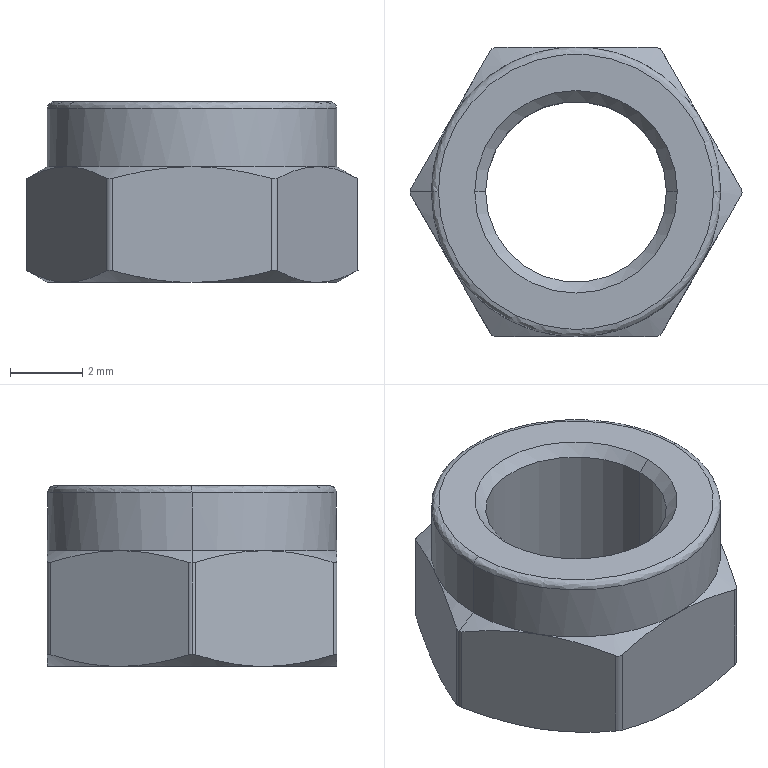Part | SolidWorks | features BaseBody 1 | 1 solid | 39 faces | box 9.176 x 8 x 5 mm | volume 166.809 mm3 | cone 18 | cylinder 11 | plane 8 | spline 2 | commonest cylinder face diameters 0.4 x7 5 x2 8 x2
STEP:
#1=CARTESIAN_POINT('',(-3.8,0.,5.));
#2=VERTEX_POINT('',#1);
#3=CARTESIAN_POINT('',(3.8,0.,5.));
#4=VERTEX_POINT('',#3);
#5=CARTESIAN_POINT('',(-3.8,0.,5.));
#6=CARTESIAN_POINT('',(-3.8,-0.2415,5.));
#7=CARTESIAN_POINT('',(-3.767,-0.5975,5.));
#8=CARTESIAN_POINT('',(-3.669,-1.002,5.));
#9=CARTESIAN_POINT('',(-3.606,-1.201,5.));
#10=CARTESIAN_POINT('',(-3.576,-1.286,5.));
#11=CARTESIAN_POINT('',(-3.555,-1.343,5.));
#12=CARTESIAN_POINT('',(-3.545,-1.369,5.));
#13=CARTESIAN_POINT('',(-3.486,-1.518,5.));
#14=CARTESIAN_POINT('',(-3.407,-1.693,5.));
#15=CARTESIAN_POINT('',(-3.314,-1.86,5.));
#16=CARTESIAN_POINT('',(-3.249,-1.971,5.));
#17=CARTESIAN_POINT('',(-3.216,-2.025,5.));
#18=CARTESIAN_POINT('',(-3.037,-2.299,5.));
#19=CARTESIAN_POINT('',(-2.872,-2.502,5.));
#20=CARTESIAN_POINT('',(-2.594,-2.78,5.));
#21=CARTESIAN_POINT('',(-2.449,-2.911,5.));
#22=CARTESIAN_POINT('',(-2.294,-3.03,5.));
#23=CARTESIAN_POINT('',(-2.188,-3.107,5.));
#24=CARTESIAN_POINT('',(-2.133,-3.145,5.));
#25=CARTESIAN_POINT('',(-1.972,-3.251,5.));
#26=CARTESIAN_POINT('',(-1.806,-3.347,5.));
#27=CARTESIAN_POINT('',(-1.605,-3.445,5.));
#28=CARTESIAN_POINT('',(-1.517,-3.484,5.));
#29=CARTESIAN_POINT('',(-1.458,-3.509,5.));
#30=CARTESIAN_POINT('',(-1.427,-3.522,5.));
#31=CARTESIAN_POINT('',(-0.9498,-3.711,5.));
#32=CARTESIAN_POINT('',(-0.4829,-3.8,5.));
#33=CARTESIAN_POINT('',(0.2414,-3.8,5.));
#34=CARTESIAN_POINT('',(0.5974,-3.767,5.));
#35=CARTESIAN_POINT('',(1.002,-3.669,5.));
#36=CARTESIAN_POINT('',(1.201,-3.606,5.));
#37=CARTESIAN_POINT('',(1.286,-3.576,5.));
#38=CARTESIAN_POINT('',(1.342,-3.555,5.));
#39=CARTESIAN_POINT('',(1.369,-3.545,5.));
#40=CARTESIAN_POINT('',(1.518,-3.486,5.));
#41=CARTESIAN_POINT('',(1.693,-3.407,5.));
#42=CARTESIAN_POINT('',(1.86,-3.314,5.));
#43=CARTESIAN_POINT('',(1.971,-3.249,5.));
#44=CARTESIAN_POINT('',(2.025,-3.216,5.));
#45=CARTESIAN_POINT('',(2.299,-3.037,5.));
#46=CARTESIAN_POINT('',(2.502,-2.872,5.));
#47=CARTESIAN_POINT('',(2.78,-2.594,5.));
#48=CARTESIAN_POINT('',(2.911,-2.449,5.));
#49=CARTESIAN_POINT('',(3.03,-2.294,5.));
#50=CARTESIAN_POINT('',(3.107,-2.188,5.));
#51=CARTESIAN_POINT('',(3.145,-2.133,5.));
#52=CARTESIAN_POINT('',(3.251,-1.972,5.));
#53=CARTESIAN_POINT('',(3.347,-1.806,5.));
#54=CARTESIAN_POINT('',(3.445,-1.605,5.));
#55=CARTESIAN_POINT('',(3.484,-1.517,5.));
#56=CARTESIAN_POINT('',(3.509,-1.458,5.));
#57=CARTESIAN_POINT('',(3.522,-1.427,5.));
#58=CARTESIAN_POINT('',(3.711,-0.9496,5.));
#59=CARTESIAN_POINT('',(3.8,-0.4834,5.));
#60=CARTESIAN_POINT('',(3.8,0.,5.));
#61=B_SPLINE_CURVE_WITH_KNOTS('',3,(#5,#6,#7,#8,#9,#10,#11,#12,#13,#14,#15,#16,#17,#18,#19,#20,#21,#22,#23,#24,#25,#26,#27,#28,#29,#30,#31,#32,#33,#34,#35,#36,#37,#38,#39,#40,#41,#42,#43,#44,#45,#46,#47,#48,#49,#50,#51,#52,#53,#54,#55,#56,#57,#58,#59,#60),.UNSPECIFIED.,.F.,.F.,(4,1,1,1,2,2,1,2,2,2,1,2,2,1,1,2,2,2,1,1,1,2,2,1,2,2,2,1,2,2,1,1,2,2,4),(0.,0.0625,0.09375,0.1094,0.1172,0.125,0.1562,0.1719,0.1875,0.25,0.2812,0.2969,0.3125,0.3437,0.3594,0.3672,0.375,0.5,0.5625,0.5937,0.6094,0.6172,0.625,0.6562,0.6719,0.6875,0.75,0.7812,0.7969,0.8125,0.8437,0.8594,0.8672,0.875,1.),.UNSPECIFIED.);
#62=EDGE_CURVE('',#2,#4,#61,.T.);
#63=ORIENTED_EDGE('',*,*,#62,.F.);
#64=CARTESIAN_POINT('',(-4.,0.,4.8));
#65=VERTEX_POINT('',#64);
#66=CARTESIAN_POINT('',(-3.8,0.,4.8));
#67=DIRECTION('',(0.,-1.,0.));
#68=DIRECTION('',(-1.,0.,0.));
#69=AXIS2_PLACEMENT_3D('',#66,#67,#68);
#70=CIRCLE('',#69,0.2);
#71=EDGE_CURVE('',#2,#65,#70,.T.);
#72=ORIENTED_EDGE('',*,*,#71,.T.);
#73=CARTESIAN_POINT('',(4.,0.,4.8));
#74=VERTEX_POINT('',#73);
#75=CARTESIAN_POINT('',(0.,0.,4.8));
#76=DIRECTION('',(0.,0.,1.));
#77=DIRECTION('',(1.,0.,0.));
#78=AXIS2_PLACEMENT_3D('',#75,#76,#77);
#79=CIRCLE('',#78,4.);
#80=EDGE_CURVE('',#65,#74,#79,.T.);
#81=ORIENTED_EDGE('',*,*,#80,.T.);
#82=CARTESIAN_POINT('',(3.8,0.,4.8));
#83=DIRECTION('',(0.,1.,0.));
#84=DIRECTION('',(1.,0.,0.));
#85=AXIS2_PLACEMENT_3D('',#82,#83,#84);
#86=CIRCLE('',#85,0.2);
#87=EDGE_CURVE('',#4,#74,#86,.T.);
#88=ORIENTED_EDGE('',*,*,#87,.F.);
#89=EDGE_LOOP('',(#63,#72,#81,#88));
#90=FACE_OUTER_BOUND('',#89,.T.);
#91=CARTESIAN_POINT('',(-3.8,0.,5.));
#92=CARTESIAN_POINT('',(-3.8,-7.6,5.));
#93=CARTESIAN_POINT('',(3.8,-7.6,5.));
#94=CARTESIAN_POINT('',(3.8,0.,5.));
#95=CARTESIAN_POINT('',(-3.917,0.,5.));
#96=CARTESIAN_POINT('',(-3.917,-7.834,5.));
#97=CARTESIAN_POINT('',(3.917,-7.834,5.));
#98=CARTESIAN_POINT('',(3.917,0.,5.));
#99=CARTESIAN_POINT('',(-4.,0.,4.917));
#100=CARTESIAN_POINT('',(-4.,-8.,4.917));
#101=CARTESIAN_POINT('',(4.,-8.,4.917));
#102=CARTESIAN_POINT('',(4.,0.,4.917));
#103=CARTESIAN_POINT('',(-4.,0.,4.8));
#104=CARTESIAN_POINT('',(-4.,-8.,4.8));
#105=CARTESIAN_POINT('',(4.,-8.,4.8));
#106=CARTESIAN_POINT('',(4.,0.,4.8));
#107=(BOUNDED_SURFACE()B_SPLINE_SURFACE(3,3,((#91,#92,#93,#94),(#95,#96,#97,#98),(#99,#100,#101,#102),(#103,#104,#105,#106)),.UNSPECIFIED.,.F.,.F.,.T.)B_SPLINE_SURFACE_WITH_KNOTS((4,4),(4,4),(0.,1.),(0.,1.),.UNSPECIFIED.)GEOMETRIC_REPRESENTATION_ITEM()RATIONAL_B_SPLINE_SURFACE(((1.,0.3333,0.3333,1.),(0.8047,0.2682,0.2682,0.8047),(0.8047,0.2682,0.2682,0.8047),(1.,0.3333,0.3333,1.)))REPRESENTATION_ITEM('')SURFACE());
#108=ADVANCED_FACE('',(#90),#107,.T.);
#109=CARTESIAN_POINT('',(-2.5,0.,0.3));
#110=VERTEX_POINT('',#109);
#111=CARTESIAN_POINT('',(2.5,0.,0.3));
#112=VERTEX_POINT('',#111);
#113=CARTESIAN_POINT('',(0.,0.,0.3));
#114=DIRECTION('',(0.,0.,1.));
#115=DIRECTION('',(1.,0.,0.));
#116=AXIS2_PLACEMENT_3D('',#113,#114,#115);
#117=CIRCLE('',#116,2.5);
#118=EDGE_CURVE('',#110,#112,#117,.T.);
#119=ORIENTED_EDGE('',*,*,#118,.F.);
#120=CARTESIAN_POINT('',(-2.5,0.,4.7));
#121=VERTEX_POINT('',#120);
#122=CARTESIAN_POINT('',(-2.5,0.,0.));
#123=DIRECTION('',(0.,0.,1.));
#124=VECTOR('',#123,1000.);
#125=LINE('',#122,#124);
#126=EDGE_CURVE('',#110,#121,#125,.T.);
#127=ORIENTED_EDGE('',*,*,#126,.T.);
#128=CARTESIAN_POINT('',(2.5,0.,4.7));
#129=VERTEX_POINT('',#128);
#130=CARTESIAN_POINT('',(0.,0.,4.7));
#131=DIRECTION('',(0.,0.,-1.));
#132=DIRECTION('',(1.,0.,0.));
#133=AXIS2_PLACEMENT_3D('',#130,#131,#132);
#134=CIRCLE('',#133,2.5);
#135=EDGE_CURVE('',#129,#121,#134,.T.);
#136=ORIENTED_EDGE('',*,*,#135,.F.);
#137=CARTESIAN_POINT('',(2.5,0.,0.));
#138=DIRECTION('',(0.,0.,1.));
#139=VECTOR('',#138,1000.);
#140=LINE('',#137,#139);
#141=EDGE_CURVE('',#112,#129,#140,.T.);
#142=ORIENTED_EDGE('',*,*,#141,.F.);
#143=EDGE_LOOP('',(#119,#127,#136,#142));
#144=FACE_OUTER_BOUND('',#143,.T.);
#145=CARTESIAN_POINT('',(0.,0.,0.));
#146=DIRECTION('',(0.,0.,1.));
#147=DIRECTION('',(1.,0.,0.));
#148=AXIS2_PLACEMENT_3D('',#145,#146,#147);
#149=CYLINDRICAL_SURFACE('',#148,2.5);
#150=ADVANCED_FACE('',(#144),#149,.F.);
#151=ORIENTED_EDGE('',*,*,#118,.T.);
#152=CARTESIAN_POINT('',(2.8,0.,0.));
#153=VERTEX_POINT('',#152);
#154=CARTESIAN_POINT('',(2.8,0.,0.));
#155=DIRECTION('',(0.7071,0.,-0.7071));
#156=VECTOR('',#155,1000.);
#157=LINE('',#154,#156);
#158=EDGE_CURVE('',#112,#153,#157,.T.);
#159=ORIENTED_EDGE('',*,*,#158,.T.);
#160=CARTESIAN_POINT('',(-2.8,0.,0.));
#161=VERTEX_POINT('',#160);
#162=CARTESIAN_POINT('',(0.,0.,0.));
#163=DIRECTION('',(0.,0.,1.));
#164=DIRECTION('',(-1.,0.,0.));
#165=AXIS2_PLACEMENT_3D('',#162,#163,#164);
#166=CIRCLE('',#165,2.8);
#167=EDGE_CURVE('',#161,#153,#166,.T.);
#168=ORIENTED_EDGE('',*,*,#167,.F.);
#169=CARTESIAN_POINT('',(-2.8,0.,0.));
#170=DIRECTION('',(-0.7071,0.,-0.7071));
#171=VECTOR('',#170,1000.);
#172=LINE('',#169,#171);
#173=EDGE_CURVE('',#110,#161,#172,.T.);
#174=ORIENTED_EDGE('',*,*,#173,.F.);
#175=EDGE_LOOP('',(#151,#159,#168,#174));
#176=FACE_OUTER_BOUND('',#175,.T.);
#177=CARTESIAN_POINT('',(0.,0.,0.));
#178=DIRECTION('',(0.,0.,-1.));
#179=DIRECTION('',(-1.,0.,0.));
#180=AXIS2_PLACEMENT_3D('',#177,#178,#179);
#181=CONICAL_SURFACE('',#180,2.8,0.7854);
#182=ADVANCED_FACE('',(#176),#181,.F.);
#183=ORIENTED_EDGE('',*,*,#135,.T.);
#184=CARTESIAN_POINT('',(-2.8,0.,5.));
#185=VERTEX_POINT('',#184);
#186=CARTESIAN_POINT('',(-2.8,0.,5.));
#187=DIRECTION('',(-0.7071,0.,0.7071));
#188=VECTOR('',#187,1000.);
#189=LINE('',#186,#188);
#190=EDGE_CURVE('',#121,#185,#189,.T.);
#191=ORIENTED_EDGE('',*,*,#190,.T.);
#192=CARTESIAN_POINT('',(2.8,0.,5.));
#193=VERTEX_POINT('',#192);
#194=CARTESIAN_POINT('',(0.,0.,5.));
#195=DIRECTION('',(0.,0.,-1.));
#196=DIRECTION('',(1.,0.,0.));
#197=AXIS2_PLACEMENT_3D('',#194,#195,#196);
#198=CIRCLE('',#197,2.8);
#199=EDGE_CURVE('',#193,#185,#198,.T.);
#200=ORIENTED_EDGE('',*,*,#199,.F.);
#201=CARTESIAN_POINT('',(2.8,0.,5.));
#202=DIRECTION('',(0.7071,0.,0.7071));
#203=VECTOR('',#202,1000.);
#204=LINE('',#201,#203);
#205=EDGE_CURVE('',#129,#193,#204,.T.);
#206=ORIENTED_EDGE('',*,*,#205,.F.);
#207=EDGE_LOOP('',(#183,#191,#200,#206));
#208=FACE_OUTER_BOUND('',#207,.T.);
#209=CARTESIAN_POINT('',(0.,0.,5.));
#210=DIRECTION('',(0.,0.,1.));
#211=DIRECTION('',(1.,0.,0.));
#212=AXIS2_PLACEMENT_3D('',#209,#210,#211);
#213=CONICAL_SURFACE('',#212,2.8,0.7854);
#214=ADVANCED_FACE('',(#208),#213,.F.);
#215=CARTESIAN_POINT('',(3.464,-2.,0.));
#216=VERTEX_POINT('',#215);
#217=CARTESIAN_POINT('',(4.,0.,0.));
#218=VERTEX_POINT('',#217);
#219=CARTESIAN_POINT('',(0.,0.,0.));
#220=DIRECTION('',(0.,0.,1.));
#221=DIRECTION('',(1.,0.,0.));
#222=AXIS2_PLACEMENT_3D('',#219,#220,#221);
#223=CIRCLE('',#222,4.);
#224=EDGE_CURVE('',#216,#218,#223,.T.);
#225=ORIENTED_EDGE('',*,*,#224,.T.);
#226=CARTESIAN_POINT('',(4.588,0.,0.3394));
#227=VERTEX_POINT('',#226);
#228=CARTESIAN_POINT('',(4.591,0.,0.3414));
#229=DIRECTION('',(0.866,0.,0.5));
#230=VECTOR('',#229,1000.);
#231=LINE('',#228,#230);
#232=EDGE_CURVE('',#218,#227,#231,.T.);
#233=ORIENTED_EDGE('',*,*,#232,.T.);
#234=CARTESIAN_POINT('',(4.561,-0.1,0.3246));
#235=VERTEX_POINT('',#234);
#236=CARTESIAN_POINT('',(4.561,-0.1,0.3246));
#237=CARTESIAN_POINT('',(4.578,-0.07028,0.3341));
#238=CARTESIAN_POINT('',(4.588,-0.03564,0.3394));
#239=CARTESIAN_POINT('',(4.588,0.,0.3394));
#240=B_SPLINE_CURVE_WITH_KNOTS('',3,(#236,#237,#238,#239),.UNSPECIFIED.,.F.,.F.,(4,4),(-0.0001053,0.),.UNSPECIFIED.);
#241=EDGE_CURVE('',#235,#227,#240,.T.);
#242=ORIENTED_EDGE('',*,*,#241,.F.);
#243=CARTESIAN_POINT('',(4.561,-0.1,0.3246));
#244=CARTESIAN_POINT('',(4.202,-0.7217,0.1253));
#245=CARTESIAN_POINT('',(3.838,-1.353,0.));
#246=CARTESIAN_POINT('',(3.464,-2.,0.));
#247=B_SPLINE_CURVE_WITH_KNOTS('',3,(#243,#244,#245,#246),.UNSPECIFIED.,.F.,.F.,(4,4),(0.,0.002218),.UNSPECIFIED.);
#248=EDGE_CURVE('',#235,#216,#247,.T.);
#249=ORIENTED_EDGE('',*,*,#248,.T.);
#250=EDGE_LOOP('',(#225,#233,#242,#249));
#251=FACE_OUTER_BOUND('',#250,.T.);
#252=CARTESIAN_POINT('',(0.,0.,0.3414));
#253=DIRECTION('',(0.,0.,1.));
#254=DIRECTION('',(1.,0.,0.));
#255=AXIS2_PLACEMENT_3D('',#252,#253,#254);
#256=CONICAL_SURFACE('',#255,4.591,1.047);
#257=ADVANCED_FACE('',(#251),#256,.T.);
#258=CARTESIAN_POINT('',(0.,0.,4.8));
#259=DIRECTION('',(0.,0.,1.));
#260=DIRECTION('',(1.,0.,0.));
#261=AXIS2_PLACEMENT_3D('',#258,#259,#260);
#262=CIRCLE('',#261,4.);
#263=EDGE_CURVE('',#74,#65,#262,.T.);
#264=ORIENTED_EDGE('',*,*,#263,.F.);
#265=CARTESIAN_POINT('',(4.,0.,3.2));
#266=VERTEX_POINT('',#265);
#267=CARTESIAN_POINT('',(4.,0.,5.));
#268=DIRECTION('',(0.,0.,-1.));
#269=VECTOR('',#268,1000.);
#270=LINE('',#267,#269);
#271=EDGE_CURVE('',#74,#266,#270,.T.);
#272=ORIENTED_EDGE('',*,*,#271,.T.);
#273=CARTESIAN_POINT('',(3.464,2.,3.2));
#274=VERTEX_POINT('',#273);
#275=CARTESIAN_POINT('',(0.,0.,3.2));
#276=DIRECTION('',(0.,0.,1.));
#277=DIRECTION('',(-1.,0.,0.));
#278=AXIS2_PLACEMENT_3D('',#275,#276,#277);
#279=CIRCLE('',#278,4.);
#280=EDGE_CURVE('',#266,#274,#279,.T.);
#281=ORIENTED_EDGE('',*,*,#280,.T.);
#282=CARTESIAN_POINT('',(0.,4.,3.2));
#283=VERTEX_POINT('',#282);
#284=CARTESIAN_POINT('',(0.,0.,3.2));
#285=DIRECTION('',(0.,0.,1.));
#286=DIRECTION('',(-1.,0.,0.));
#287=AXIS2_PLACEMENT_3D('',#284,#285,#286);
#288=CIRCLE('',#287,4.);
#289=EDGE_CURVE('',#274,#283,#288,.T.);
#290=ORIENTED_EDGE('',*,*,#289,.T.);
#291=CARTESIAN_POINT('',(-3.464,2.,3.2));
#292=VERTEX_POINT('',#291);
#293=CARTESIAN_POINT('',(0.,0.,3.2));
#294=DIRECTION('',(0.,0.,1.));
#295=DIRECTION('',(-1.,0.,0.));
#296=AXIS2_PLACEMENT_3D('',#293,#294,#295);
#297=CIRCLE('',#296,4.);
#298=EDGE_CURVE('',#283,#292,#297,.T.);
#299=ORIENTED_EDGE('',*,*,#298,.T.);
#300=CARTESIAN_POINT('',(-4.,0.,3.2));
#301=VERTEX_POINT('',#300);
#302=CARTESIAN_POINT('',(0.,0.,3.2));
#303=DIRECTION('',(0.,0.,1.));
#304=DIRECTION('',(-1.,0.,0.));
#305=AXIS2_PLACEMENT_3D('',#302,#303,#304);
#306=CIRCLE('',#305,4.);
#307=EDGE_CURVE('',#292,#301,#306,.T.);
#308=ORIENTED_EDGE('',*,*,#307,.T.);
#309=CARTESIAN_POINT('',(-4.,0.,5.));
#310=DIRECTION('',(0.,0.,-1.));
#311=VECTOR('',#310,1000.);
#312=LINE('',#309,#311);
#313=EDGE_CURVE('',#65,#301,#312,.T.);
#314=ORIENTED_EDGE('',*,*,#313,.F.);
#315=EDGE_LOOP('',(#264,#272,#281,#290,#299,#308,#314));
#316=FACE_OUTER_BOUND('',#315,.T.);
#317=CARTESIAN_POINT('',(0.,0.,5.));
#318=DIRECTION('',(0.,0.,-1.));
#319=DIRECTION('',(-1.,0.,0.));
#320=AXIS2_PLACEMENT_3D('',#317,#318,#319);
#321=CYLINDRICAL_SURFACE('',#320,4.);
#322=ADVANCED_FACE('',(#316),#321,.T.);
#323=CARTESIAN_POINT('',(-3.464,-2.,3.2));
#324=VERTEX_POINT('',#323);
#325=CARTESIAN_POINT('',(0.,0.,3.2));
#326=DIRECTION('',(0.,0.,1.));
#327=DIRECTION('',(-1.,0.,0.));
#328=AXIS2_PLACEMENT_3D('',#325,#326,#327);
#329=CIRCLE('',#328,4.);
#330=EDGE_CURVE('',#301,#324,#329,.T.);
#331=ORIENTED_EDGE('',*,*,#330,.F.);
#332=CARTESIAN_POINT('',(-4.588,0.,2.861));
#333=VERTEX_POINT('',#332);
#334=CARTESIAN_POINT('',(-4.591,0.,2.859));
#335=DIRECTION('',(-0.866,0.,-0.5));
#336=VECTOR('',#335,1000.);
#337=LINE('',#334,#336);
#338=EDGE_CURVE('',#301,#333,#337,.T.);
#339=ORIENTED_EDGE('',*,*,#338,.T.);
#340=CARTESIAN_POINT('',(-4.561,-0.1,2.875));
#341=VERTEX_POINT('',#340);
#342=CARTESIAN_POINT('',(-4.588,0.,2.861));
#343=CARTESIAN_POINT('',(-4.588,-0.03565,2.861));
#344=CARTESIAN_POINT('',(-4.578,-0.07027,2.866));
#345=CARTESIAN_POINT('',(-4.561,-0.1,2.875));
#346=B_SPLINE_CURVE_WITH_KNOTS('',3,(#342,#343,#344,#345),.UNSPECIFIED.,.F.,.F.,(4,4),(0.,0.0001053),.UNSPECIFIED.);
#347=EDGE_CURVE('',#333,#341,#346,.T.);
#348=ORIENTED_EDGE('',*,*,#347,.T.);
#349=CARTESIAN_POINT('',(-4.561,-0.1,2.875));
#350=CARTESIAN_POINT('',(-4.202,-0.7217,3.075));
#351=CARTESIAN_POINT('',(-3.838,-1.353,3.2));
#352=CARTESIAN_POINT('',(-3.464,-2.,3.2));
#353=B_SPLINE_CURVE_WITH_KNOTS('',3,(#349,#350,#351,#352),.UNSPECIFIED.,.F.,.F.,(4,4),(0.,0.002218),.UNSPECIFIED.);
#354=EDGE_CURVE('',#341,#324,#353,.T.);
#355=ORIENTED_EDGE('',*,*,#354,.T.);
#356=EDGE_LOOP('',(#331,#339,#348,#355));
#357=FACE_OUTER_BOUND('',#356,.T.);
#358=CARTESIAN_POINT('',(0.,0.,2.859));
#359=DIRECTION('',(0.,0.,-1.));
#360=DIRECTION('',(-1.,0.,0.));
#361=AXIS2_PLACEMENT_3D('',#358,#359,#360);
#362=CONICAL_SURFACE('',#361,4.591,1.047);
#363=ADVANCED_FACE('',(#357),#362,.T.);
#364=ORIENTED_EDGE('',*,*,#347,.F.);
#365=CARTESIAN_POINT('',(-4.588,0.,0.3394));
#366=VERTEX_POINT('',#365);
#367=CARTESIAN_POINT('',(-4.588,0.,3.2));
#368=DIRECTION('',(0.,0.,-1.));
#369=VECTOR('',#368,1000.);
#370=LINE('',#367,#369);
#371=EDGE_CURVE('',#333,#366,#370,.T.);
#372=ORIENTED_EDGE('',*,*,#371,.T.);
#373=CARTESIAN_POINT('',(-4.561,-0.1,0.3246));
#374=VERTEX_POINT('',#373);
#375=CARTESIAN_POINT('',(-4.588,0.,0.3394));
#376=CARTESIAN_POINT('',(-4.588,-0.03565,0.3394));
#377=CARTESIAN_POINT('',(-4.578,-0.07027,0.3341));
#378=CARTESIAN_POINT('',(-4.561,-0.1,0.3246));
#379=B_SPLINE_CURVE_WITH_KNOTS('',3,(#375,#376,#377,#378),.UNSPECIFIED.,.F.,.F.,(4,4),(0.,0.0001053),.UNSPECIFIED.);
#380=EDGE_CURVE('',#366,#374,#379,.T.);
#381=ORIENTED_EDGE('',*,*,#380,.T.);
#382=CARTESIAN_POINT('',(-4.561,-0.1,3.2));
#383=DIRECTION('',(0.,0.,1.));
#384=VECTOR('',#383,1000.);
#385=LINE('',#382,#384);
#386=EDGE_CURVE('',#374,#341,#385,.T.);
#387=ORIENTED_EDGE('',*,*,#386,.T.);
#388=EDGE_LOOP('',(#364,#372,#381,#387));
#389=FACE_OUTER_BOUND('',#388,.T.);
#390=CARTESIAN_POINT('',(-4.388,0.,3.2));
#391=DIRECTION('',(0.,0.,-1.));
#392=DIRECTION('',(-1.,0.,0.));
#393=AXIS2_PLACEMENT_3D('',#390,#391,#392);
#394=CYLINDRICAL_SURFACE('',#393,0.2);
#395=ADVANCED_FACE('',(#389),#394,.T.);
#396=ORIENTED_EDGE('',*,*,#126,.F.);
#397=CARTESIAN_POINT('',(0.,0.,0.3));
#398=DIRECTION('',(0.,0.,1.));
#399=DIRECTION('',(1.,0.,0.));
#400=AXIS2_PLACEMENT_3D('',#397,#398,#399);
#401=CIRCLE('',#400,2.5);
#402=EDGE_CURVE('',#112,#110,#401,.T.);
#403=ORIENTED_EDGE('',*,*,#402,.F.);
#404=ORIENTED_EDGE('',*,*,#141,.T.);
#405=CARTESIAN_POINT('',(0.,0.,4.7));
#406=DIRECTION('',(0.,0.,-1.));
#407=DIRECTION('',(1.,0.,0.));
#408=AXIS2_PLACEMENT_3D('',#405,#406,#407);
#409=CIRCLE('',#408,2.5);
#410=EDGE_CURVE('',#121,#129,#409,.T.);
#411=ORIENTED_EDGE('',*,*,#410,.F.);
#412=EDGE_LOOP('',(#396,#403,#404,#411));
#413=FACE_OUTER_BOUND('',#412,.T.);
#414=CARTESIAN_POINT('',(0.,0.,0.));
#415=DIRECTION('',(0.,0.,1.));
#416=DIRECTION('',(1.,0.,0.));
#417=AXIS2_PLACEMENT_3D('',#414,#415,#416);
#418=CYLINDRICAL_SURFACE('',#417,2.5);
#419=ADVANCED_FACE('',(#413),#418,.F.);
#420=ORIENTED_EDGE('',*,*,#158,.F.);
#421=ORIENTED_EDGE('',*,*,#402,.T.);
#422=ORIENTED_EDGE('',*,*,#173,.T.);
#423=CARTESIAN_POINT('',(0.,0.,0.));
#424=DIRECTION('',(0.,0.,1.));
#425=DIRECTION('',(-1.,0.,0.));
#426=AXIS2_PLACEMENT_3D('',#423,#424,#425);
#427=CIRCLE('',#426,2.8);
#428=EDGE_CURVE('',#153,#161,#427,.T.);
#429=ORIENTED_EDGE('',*,*,#428,.F.);
#430=EDGE_LOOP('',(#420,#421,#422,#429));
#431=FACE_OUTER_BOUND('',#430,.T.);
#432=CARTESIAN_POINT('',(0.,0.,0.));
#433=DIRECTION('',(0.,0.,-1.));
#434=DIRECTION('',(-1.,0.,0.));
#435=AXIS2_PLACEMENT_3D('',#432,#433,#434);
#436=CONICAL_SURFACE('',#435,2.8,0.7854);
#437=ADVANCED_FACE('',(#431),#436,.F.);
#438=ORIENTED_EDGE('',*,*,#190,.F.);
#439=ORIENTED_EDGE('',*,*,#410,.T.);
#440=ORIENTED_EDGE('',*,*,#205,.T.);
#441=CARTESIAN_POINT('',(0.,0.,5.));
#442=DIRECTION('',(0.,0.,-1.));
#443=DIRECTION('',(1.,0.,0.));
#444=AXIS2_PLACEMENT_3D('',#441,#442,#443);
#445=CIRCLE('',#444,2.8);
#446=EDGE_CURVE('',#185,#193,#445,.T.);
#447=ORIENTED_EDGE('',*,*,#446,.F.);
#448=EDGE_LOOP('',(#438,#439,#440,#447));
#449=FACE_OUTER_BOUND('',#448,.T.);
#450=CARTESIAN_POINT('',(0.,0.,5.));
#451=DIRECTION('',(0.,0.,1.));
#452=DIRECTION('',(1.,0.,0.));
#453=AXIS2_PLACEMENT_3D('',#450,#451,#452);
#454=CONICAL_SURFACE('',#453,2.8,0.7854);
#455=ADVANCED_FACE('',(#449),#454,.F.);
#456=ORIENTED_EDGE('',*,*,#224,.F.);
#457=CARTESIAN_POINT('',(0.,-4.,0.));
#458=VERTEX_POINT('',#457);
#459=CARTESIAN_POINT('',(0.,0.,0.));
#460=DIRECTION('',(0.,0.,1.));
#461=DIRECTION('',(1.,0.,0.));
#462=AXIS2_PLACEMENT_3D('',#459,#460,#461);
#463=CIRCLE('',#462,4.);
#464=EDGE_CURVE('',#458,#216,#463,.T.);
#465=ORIENTED_EDGE('',*,*,#464,.F.);
#466=CARTESIAN_POINT('',(-3.464,-2.,0.));
#467=VERTEX_POINT('',#466);
#468=CARTESIAN_POINT('',(0.,0.,0.));
#469=DIRECTION('',(0.,0.,1.));
#470=DIRECTION('',(1.,0.,0.));
#471=AXIS2_PLACEMENT_3D('',#468,#469,#470);
#472=CIRCLE('',#471,4.);
#473=EDGE_CURVE('',#467,#458,#472,.T.);
#474=ORIENTED_EDGE('',*,*,#473,.F.);
#475=CARTESIAN_POINT('',(-3.464,2.,0.));
#476=VERTEX_POINT('',#475);
#477=CARTESIAN_POINT('',(0.,0.,0.));
#478=DIRECTION('',(0.,0.,1.));
#479=DIRECTION('',(1.,0.,0.));
#480=AXIS2_PLACEMENT_3D('',#477,#478,#479);
#481=CIRCLE('',#480,4.);
#482=EDGE_CURVE('',#476,#467,#481,.T.);
#483=ORIENTED_EDGE('',*,*,#482,.F.);
#484=CARTESIAN_POINT('',(0.,4.,0.));
#485=VERTEX_POINT('',#484);
#486=CARTESIAN_POINT('',(0.,0.,0.));
#487=DIRECTION('',(0.,0.,1.));
#488=DIRECTION('',(1.,0.,0.));
#489=AXIS2_PLACEMENT_3D('',#486,#487,#488);
#490=CIRCLE('',#489,4.);
#491=EDGE_CURVE('',#485,#476,#490,.T.);
#492=ORIENTED_EDGE('',*,*,#491,.F.);
#493=CARTESIAN_POINT('',(3.464,2.,0.));
#494=VERTEX_POINT('',#493);
#495=CARTESIAN_POINT('',(0.,0.,0.));
#496=DIRECTION('',(0.,0.,1.));
#497=DIRECTION('',(1.,0.,0.));
#498=AXIS2_PLACEMENT_3D('',#495,#496,#497);
#499=CIRCLE('',#498,4.);
#500=EDGE_CURVE('',#494,#485,#499,.T.);
#501=ORIENTED_EDGE('',*,*,#500,.F.);
#502=CARTESIAN_POINT('',(0.,0.,0.));
#503=DIRECTION('',(0.,0.,1.));
#504=DIRECTION('',(1.,0.,0.));
#505=AXIS2_PLACEMENT_3D('',#502,#503,#504);
#506=CIRCLE('',#505,4.);
#507=EDGE_CURVE('',#218,#494,#506,.T.);
#508=ORIENTED_EDGE('',*,*,#507,.F.);
#509=EDGE_LOOP('',(#456,#465,#474,#483,#492,#501,#508));
#510=FACE_OUTER_BOUND('',#509,.T.);
#511=ORIENTED_EDGE('',*,*,#167,.T.);
#512=ORIENTED_EDGE('',*,*,#428,.T.);
#513=EDGE_LOOP('',(#511,#512));
#514=FACE_BOUND('',#513,.T.);
#515=CARTESIAN_POINT('',(0.,0.,0.));
#516=DIRECTION('',(0.,0.,1.));
#517=DIRECTION('',(1.,0.,0.));
#518=AXIS2_PLACEMENT_3D('',#515,#516,#517);
#519=PLANE('',#518);
#520=ADVANCED_FACE('',(#510,#514),#519,.F.);
#521=ORIENTED_EDGE('',*,*,#199,.T.);
#522=ORIENTED_EDGE('',*,*,#446,.T.);
#523=EDGE_LOOP('',(#521,#522));
#524=FACE_BOUND('',#523,.T.);
#525=CARTESIAN_POINT('',(3.8,0.,5.));
#526=CARTESIAN_POINT('',(3.8,0.2415,5.));
#527=CARTESIAN_POINT('',(3.767,0.5975,5.));
#528=CARTESIAN_POINT('',(3.669,1.002,5.));
#529=CARTESIAN_POINT('',(3.606,1.201,5.));
#530=CARTESIAN_POINT('',(3.576,1.286,5.));
#531=CARTESIAN_POINT('',(3.555,1.343,5.));
#532=CARTESIAN_POINT('',(3.545,1.369,5.));
#533=CARTESIAN_POINT('',(3.486,1.518,5.));
#534=CARTESIAN_POINT('',(3.407,1.693,5.));
#535=CARTESIAN_POINT('',(3.314,1.86,5.));
#536=CARTESIAN_POINT('',(3.249,1.971,5.));
#537=CARTESIAN_POINT('',(3.216,2.025,5.));
#538=CARTESIAN_POINT('',(3.037,2.299,5.));
#539=CARTESIAN_POINT('',(2.872,2.502,5.));
#540=CARTESIAN_POINT('',(2.594,2.78,5.));
#541=CARTESIAN_POINT('',(2.449,2.911,5.));
#542=CARTESIAN_POINT('',(2.294,3.03,5.));
#543=CARTESIAN_POINT('',(2.188,3.107,5.));
#544=CARTESIAN_POINT('',(2.133,3.145,5.));
#545=CARTESIAN_POINT('',(1.972,3.251,5.));
#546=CARTESIAN_POINT('',(1.806,3.347,5.));
#547=CARTESIAN_POINT('',(1.605,3.445,5.));
#548=CARTESIAN_POINT('',(1.517,3.484,5.));
#549=CARTESIAN_POINT('',(1.458,3.509,5.));
#550=CARTESIAN_POINT('',(1.427,3.522,5.));
#551=CARTESIAN_POINT('',(0.9498,3.711,5.));
#552=CARTESIAN_POINT('',(0.4829,3.8,5.));
#553=CARTESIAN_POINT('',(-0.2414,3.8,5.));
#554=CARTESIAN_POINT('',(-0.5974,3.767,5.));
#555=CARTESIAN_POINT('',(-1.002,3.669,5.));
#556=CARTESIAN_POINT('',(-1.201,3.606,5.));
#557=CARTESIAN_POINT('',(-1.286,3.576,5.));
#558=CARTESIAN_POINT('',(-1.342,3.555,5.));
#559=CARTESIAN_POINT('',(-1.369,3.545,5.));
#560=CARTESIAN_POINT('',(-1.518,3.486,5.));
#561=CARTESIAN_POINT('',(-1.693,3.407,5.));
#562=CARTESIAN_POINT('',(-1.86,3.314,5.));
#563=CARTESIAN_POINT('',(-1.971,3.249,5.));
#564=CARTESIAN_POINT('',(-2.025,3.216,5.));
#565=CARTESIAN_POINT('',(-2.299,3.037,5.));
#566=CARTESIAN_POINT('',(-2.502,2.872,5.));
#567=CARTESIAN_POINT('',(-2.78,2.594,5.));
#568=CARTESIAN_POINT('',(-2.911,2.449,5.));
#569=CARTESIAN_POINT('',(-3.03,2.294,5.));
#570=CARTESIAN_POINT('',(-3.107,2.188,5.));
#571=CARTESIAN_POINT('',(-3.145,2.133,5.));
#572=CARTESIAN_POINT('',(-3.251,1.972,5.));
#573=CARTESIAN_POINT('',(-3.347,1.806,5.));
#574=CARTESIAN_POINT('',(-3.445,1.605,5.));
#575=CARTESIAN_POINT('',(-3.484,1.517,5.));
#576=CARTESIAN_POINT('',(-3.509,1.458,5.));
#577=CARTESIAN_POINT('',(-3.522,1.427,5.));
#578=CARTESIAN_POINT('',(-3.711,0.9496,5.));
#579=CARTESIAN_POINT('',(-3.8,0.4834,5.));
#580=CARTESIAN_POINT('',(-3.8,0.,5.));
#581=B_SPLINE_CURVE_WITH_KNOTS('',3,(#525,#526,#527,#528,#529,#530,#531,#532,#533,#534,#535,#536,#537,#538,#539,#540,#541,#542,#543,#544,#545,#546,#547,#548,#549,#550,#551,#552,#553,#554,#555,#556,#557,#558,#559,#560,#561,#562,#563,#564,#565,#566,#567,#568,#569,#570,#571,#572,#573,#574,#575,#576,#577,#578,#579,#580),.UNSPECIFIED.,.F.,.F.,(4,1,1,1,2,2,1,2,2,2,1,2,2,1,1,2,2,2,1,1,1,2,2,1,2,2,2,1,2,2,1,1,2,2,4),(0.,0.0625,0.09375,0.1094,0.1172,0.125,0.1562,0.1719,0.1875,0.25,0.2812,0.2969,0.3125,0.3437,0.3594,0.3672,0.375,0.5,0.5625,0.5937,0.6094,0.6172,0.625,0.6562,0.6719,0.6875,0.75,0.7812,0.7969,0.8125,0.8437,0.8594,0.8672,0.875,1.),.UNSPECIFIED.);
#582=EDGE_CURVE('',#4,#2,#581,.T.);
#583=ORIENTED_EDGE('',*,*,#582,.T.);
#584=ORIENTED_EDGE('',*,*,#62,.T.);
#585=EDGE_LOOP('',(#583,#584));
#586=FACE_OUTER_BOUND('',#585,.T.);
#587=CARTESIAN_POINT('',(0.,0.,5.));
#588=DIRECTION('',(0.,0.,1.));
#589=DIRECTION('',(1.,0.,0.));
#590=AXIS2_PLACEMENT_3D('',#587,#588,#589);
#591=PLANE('',#590);
#592=ADVANCED_FACE('',(#524,#586),#591,.T.);
#593=ORIENTED_EDGE('',*,*,#232,.F.);
#594=ORIENTED_EDGE('',*,*,#507,.T.);
#595=CARTESIAN_POINT('',(4.561,0.1,0.3246));
#596=VERTEX_POINT('',#595);
#597=CARTESIAN_POINT('',(3.464,2.,0.));
#598=CARTESIAN_POINT('',(3.838,1.353,0.));
#599=CARTESIAN_POINT('',(4.202,0.7217,0.1253));
#600=CARTESIAN_POINT('',(4.561,0.1,0.3246));
#601=B_SPLINE_CURVE_WITH_KNOTS('',3,(#597,#598,#599,#600),.UNSPECIFIED.,.F.,.F.,(4,4),(0.,0.002218),.UNSPECIFIED.);
#602=EDGE_CURVE('',#494,#596,#601,.T.);
#603=ORIENTED_EDGE('',*,*,#602,.T.);
#604=CARTESIAN_POINT('',(4.588,0.,0.3394));
#605=CARTESIAN_POINT('',(4.588,0.03565,0.3394));
#606=CARTESIAN_POINT('',(4.578,0.07027,0.3341));
#607=CARTESIAN_POINT('',(4.561,0.1,0.3246));
#608=B_SPLINE_CURVE_WITH_KNOTS('',3,(#604,#605,#606,#607),.UNSPECIFIED.,.F.,.F.,(4,4),(0.,0.0001053),.UNSPECIFIED.);
#609=EDGE_CURVE('',#227,#596,#608,.T.);
#610=ORIENTED_EDGE('',*,*,#609,.F.);
#611=EDGE_LOOP('',(#593,#594,#603,#610));
#612=FACE_OUTER_BOUND('',#611,.T.);
#613=CARTESIAN_POINT('',(0.,0.,0.3414));
#614=DIRECTION('',(0.,0.,1.));
#615=DIRECTION('',(1.,0.,0.));
#616=AXIS2_PLACEMENT_3D('',#613,#614,#615);
#617=CONICAL_SURFACE('',#616,4.591,1.047);
#618=ADVANCED_FACE('',(#612),#617,.T.);
#619=ORIENTED_EDGE('',*,*,#464,.T.);
#620=CARTESIAN_POINT('',(2.367,-3.9,0.3246));
#621=VERTEX_POINT('',#620);
#622=CARTESIAN_POINT('',(3.464,-2.,0.));
#623=CARTESIAN_POINT('',(3.09,-2.647,0.));
#624=CARTESIAN_POINT('',(2.726,-3.278,0.1253));
#625=CARTESIAN_POINT('',(2.367,-3.9,0.3246));
#626=B_SPLINE_CURVE_WITH_KNOTS('',3,(#622,#623,#624,#625),.UNSPECIFIED.,.F.,.F.,(4,4),(0.,0.002218),.UNSPECIFIED.);
#627=EDGE_CURVE('',#216,#621,#626,.T.);
#628=ORIENTED_EDGE('',*,*,#627,.T.);
#629=CARTESIAN_POINT('',(2.194,-4.,0.3246));
#630=VERTEX_POINT('',#629);
#631=CARTESIAN_POINT('',(2.194,-4.,0.3246));
#632=CARTESIAN_POINT('',(2.228,-4.,0.3341));
#633=CARTESIAN_POINT('',(2.263,-3.991,0.3394));
#634=CARTESIAN_POINT('',(2.324,-3.956,0.3394));
#635=CARTESIAN_POINT('',(2.35,-3.93,0.3341));
#636=CARTESIAN_POINT('',(2.367,-3.9,0.3246));
#637=B_SPLINE_CURVE_WITH_KNOTS('',3,(#631,#632,#633,#634,#635,#636),.UNSPECIFIED.,.F.,.F.,(4,2,4),(0.,0.0001055,0.000211),.UNSPECIFIED.);
#638=EDGE_CURVE('',#630,#621,#637,.T.);
#639=ORIENTED_EDGE('',*,*,#638,.F.);
#640=CARTESIAN_POINT('',(2.194,-4.,0.3246));
#641=CARTESIAN_POINT('',(1.476,-4.,0.1253));
#642=CARTESIAN_POINT('',(0.7473,-4.,0.));
#643=CARTESIAN_POINT('',(0.,-4.,0.));
#644=B_SPLINE_CURVE_WITH_KNOTS('',3,(#640,#641,#642,#643),.UNSPECIFIED.,.F.,.F.,(4,4),(0.,0.002218),.UNSPECIFIED.);
#645=EDGE_CURVE('',#630,#458,#644,.T.);
#646=ORIENTED_EDGE('',*,*,#645,.T.);
#647=EDGE_LOOP('',(#619,#628,#639,#646));
#648=FACE_OUTER_BOUND('',#647,.T.);
#649=CARTESIAN_POINT('',(0.,0.,0.3415));
#650=DIRECTION('',(0.,0.,1.));
#651=DIRECTION('',(1.,0.,0.));
#652=AXIS2_PLACEMENT_3D('',#649,#650,#651);
#653=CONICAL_SURFACE('',#652,4.591,1.047);
#654=ADVANCED_FACE('',(#648),#653,.T.);
#655=CARTESIAN_POINT('',(-2.367,-3.9,0.3246));
#656=VERTEX_POINT('',#655);
#657=CARTESIAN_POINT('',(-2.194,-4.,0.3246));
#658=VERTEX_POINT('',#657);
#659=CARTESIAN_POINT('',(-2.367,-3.9,0.3246));
#660=CARTESIAN_POINT('',(-2.35,-3.93,0.3341));
#661=CARTESIAN_POINT('',(-2.325,-3.955,0.3394));
#662=CARTESIAN_POINT('',(-2.264,-3.991,0.3394));
#663=CARTESIAN_POINT('',(-2.228,-4.,0.3341));
#664=CARTESIAN_POINT('',(-2.194,-4.,0.3246));
#665=B_SPLINE_CURVE_WITH_KNOTS('',3,(#659,#660,#661,#662,#663,#664),.UNSPECIFIED.,.F.,.F.,(4,2,4),(0.,0.0001055,0.000211),.UNSPECIFIED.);
#666=EDGE_CURVE('',#656,#658,#665,.T.);
#667=ORIENTED_EDGE('',*,*,#666,.F.);
#668=CARTESIAN_POINT('',(-2.367,-3.9,0.3246));
#669=CARTESIAN_POINT('',(-2.726,-3.278,0.1253));
#670=CARTESIAN_POINT('',(-3.09,-2.647,0.));
#671=CARTESIAN_POINT('',(-3.464,-2.,0.));
#672=B_SPLINE_CURVE_WITH_KNOTS('',3,(#668,#669,#670,#671),.UNSPECIFIED.,.F.,.F.,(4,4),(0.,0.002218),.UNSPECIFIED.);
#673=EDGE_CURVE('',#656,#467,#672,.T.);
#674=ORIENTED_EDGE('',*,*,#673,.T.);
#675=ORIENTED_EDGE('',*,*,#473,.T.);
#676=CARTESIAN_POINT('',(0.,-4.,0.));
#677=CARTESIAN_POINT('',(-0.7473,-4.,0.));
#678=CARTESIAN_POINT('',(-1.476,-4.,0.1253));
#679=CARTESIAN_POINT('',(-2.194,-4.,0.3246));
#680=B_SPLINE_CURVE_WITH_KNOTS('',3,(#676,#677,#678,#679),.UNSPECIFIED.,.F.,.F.,(4,4),(0.,0.002218),.UNSPECIFIED.);
#681=EDGE_CURVE('',#458,#658,#680,.T.);
#682=ORIENTED_EDGE('',*,*,#681,.T.);
#683=EDGE_LOOP('',(#667,#674,#675,#682));
#684=FACE_OUTER_BOUND('',#683,.T.);
#685=CARTESIAN_POINT('',(0.,0.,0.3415));
#686=DIRECTION('',(0.,0.,1.));
#687=DIRECTION('',(1.,0.,0.));
#688=AXIS2_PLACEMENT_3D('',#685,#686,#687);
#689=CONICAL_SURFACE('',#688,4.591,1.047);
#690=ADVANCED_FACE('',(#684),#689,.T.);
#691=CARTESIAN_POINT('',(-4.561,0.1,0.3246));
#692=VERTEX_POINT('',#691);
#693=CARTESIAN_POINT('',(-4.561,0.1,0.3246));
#694=CARTESIAN_POINT('',(-4.578,0.07028,0.3341));
#695=CARTESIAN_POINT('',(-4.588,0.03564,0.3394));
#696=CARTESIAN_POINT('',(-4.588,0.,0.3394));
#697=B_SPLINE_CURVE_WITH_KNOTS('',3,(#693,#694,#695,#696),.UNSPECIFIED.,.F.,.F.,(4,4),(-0.0001053,0.),.UNSPECIFIED.);
#698=EDGE_CURVE('',#692,#366,#697,.T.);
#699=ORIENTED_EDGE('',*,*,#698,.F.);
#700=CARTESIAN_POINT('',(-4.561,0.1,0.3246));
#701=CARTESIAN_POINT('',(-4.202,0.7217,0.1253));
#702=CARTESIAN_POINT('',(-3.838,1.353,0.));
#703=CARTESIAN_POINT('',(-3.464,2.,0.));
#704=B_SPLINE_CURVE_WITH_KNOTS('',3,(#700,#701,#702,#703),.UNSPECIFIED.,.F.,.F.,(4,4),(0.,0.002218),.UNSPECIFIED.);
#705=EDGE_CURVE('',#692,#476,#704,.T.);
#706=ORIENTED_EDGE('',*,*,#705,.T.);
#707=ORIENTED_EDGE('',*,*,#482,.T.);
#708=CARTESIAN_POINT('',(-3.464,-2.,0.));
#709=CARTESIAN_POINT('',(-3.838,-1.353,0.));
#710=CARTESIAN_POINT('',(-4.202,-0.7217,0.1253));
#711=CARTESIAN_POINT('',(-4.561,-0.1,0.3246));
#712=B_SPLINE_CURVE_WITH_KNOTS('',3,(#708,#709,#710,#711),.UNSPECIFIED.,.F.,.F.,(4,4),(0.,0.002218),.UNSPECIFIED.);
#713=EDGE_CURVE('',#467,#374,#712,.T.);
#714=ORIENTED_EDGE('',*,*,#713,.T.);
#715=ORIENTED_EDGE('',*,*,#380,.F.);
#716=EDGE_LOOP('',(#699,#706,#707,#714,#715));
#717=FACE_OUTER_BOUND('',#716,.T.);
#718=CARTESIAN_POINT('',(0.,0.,0.3414));
#719=DIRECTION('',(0.,0.,1.));
#720=DIRECTION('',(1.,0.,0.));
#721=AXIS2_PLACEMENT_3D('',#718,#719,#720);
#722=CONICAL_SURFACE('',#721,4.591,1.047);
#723=ADVANCED_FACE('',(#717),#722,.T.);
#724=CARTESIAN_POINT('',(-2.194,4.,0.3246));
#725=VERTEX_POINT('',#724);
#726=CARTESIAN_POINT('',(-2.367,3.9,0.3246));
#727=VERTEX_POINT('',#726);
#728=CARTESIAN_POINT('',(-2.194,4.,0.3246));
#729=CARTESIAN_POINT('',(-2.228,4.,0.3341));
#730=CARTESIAN_POINT('',(-2.263,3.991,0.3394));
#731=CARTESIAN_POINT('',(-2.324,3.956,0.3394));
#732=CARTESIAN_POINT('',(-2.35,3.93,0.3341));
#733=CARTESIAN_POINT('',(-2.367,3.9,0.3246));
#734=B_SPLINE_CURVE_WITH_KNOTS('',3,(#728,#729,#730,#731,#732,#733),.UNSPECIFIED.,.F.,.F.,(4,2,4),(0.,0.0001055,0.000211),.UNSPECIFIED.);
#735=EDGE_CURVE('',#725,#727,#734,.T.);
#736=ORIENTED_EDGE('',*,*,#735,.F.);
#737=CARTESIAN_POINT('',(-2.194,4.,0.3246));
#738=CARTESIAN_POINT('',(-1.476,4.,0.1253));
#739=CARTESIAN_POINT('',(-0.7473,4.,0.));
#740=CARTESIAN_POINT('',(0.,4.,0.));
#741=B_SPLINE_CURVE_WITH_KNOTS('',3,(#737,#738,#739,#740),.UNSPECIFIED.,.F.,.F.,(4,4),(0.,0.002218),.UNSPECIFIED.);
#742=EDGE_CURVE('',#725,#485,#741,.T.);
#743=ORIENTED_EDGE('',*,*,#742,.T.);
#744=ORIENTED_EDGE('',*,*,#491,.T.);
#745=CARTESIAN_POINT('',(-3.464,2.,0.));
#746=CARTESIAN_POINT('',(-3.09,2.647,0.));
#747=CARTESIAN_POINT('',(-2.726,3.278,0.1253));
#748=CARTESIAN_POINT('',(-2.367,3.9,0.3246));
#749=B_SPLINE_CURVE_WITH_KNOTS('',3,(#745,#746,#747,#748),.UNSPECIFIED.,.F.,.F.,(4,4),(0.,0.002218),.UNSPECIFIED.);
#750=EDGE_CURVE('',#476,#727,#749,.T.);
#751=ORIENTED_EDGE('',*,*,#750,.T.);
#752=EDGE_LOOP('',(#736,#743,#744,#751));
#753=FACE_OUTER_BOUND('',#752,.T.);
#754=CARTESIAN_POINT('',(0.,0.,0.3415));
#755=DIRECTION('',(0.,0.,1.));
#756=DIRECTION('',(1.,0.,0.));
#757=AXIS2_PLACEMENT_3D('',#754,#755,#756);
#758=CONICAL_SURFACE('',#757,4.591,1.047);
#759=ADVANCED_FACE('',(#753),#758,.T.);
#760=ORIENTED_EDGE('',*,*,#500,.T.);
#761=CARTESIAN_POINT('',(2.194,4.,0.3246));
#762=VERTEX_POINT('',#761);
#763=CARTESIAN_POINT('',(0.,4.,0.));
#764=CARTESIAN_POINT('',(0.7473,4.,0.));
#765=CARTESIAN_POINT('',(1.476,4.,0.1253));
#766=CARTESIAN_POINT('',(2.194,4.,0.3246));
#767=B_SPLINE_CURVE_WITH_KNOTS('',3,(#763,#764,#765,#766),.UNSPECIFIED.,.F.,.F.,(4,4),(0.,0.002218),.UNSPECIFIED.);
#768=EDGE_CURVE('',#485,#762,#767,.T.);
#769=ORIENTED_EDGE('',*,*,#768,.T.);
#770=CARTESIAN_POINT('',(2.367,3.9,0.3246));
#771=VERTEX_POINT('',#770);
#772=CARTESIAN_POINT('',(2.367,3.9,0.3246));
#773=CARTESIAN_POINT('',(2.35,3.93,0.3341));
#774=CARTESIAN_POINT('',(2.325,3.955,0.3394));
#775=CARTESIAN_POINT('',(2.264,3.991,0.3394));
#776=CARTESIAN_POINT('',(2.228,4.,0.3341));
#777=CARTESIAN_POINT('',(2.194,4.,0.3246));
#778=B_SPLINE_CURVE_WITH_KNOTS('',3,(#772,#773,#774,#775,#776,#777),.UNSPECIFIED.,.F.,.F.,(4,2,4),(0.,0.0001055,0.000211),.UNSPECIFIED.);
#779=EDGE_CURVE('',#771,#762,#778,.T.);
#780=ORIENTED_EDGE('',*,*,#779,.F.);
#781=CARTESIAN_POINT('',(2.367,3.9,0.3246));
#782=CARTESIAN_POINT('',(2.726,3.278,0.1253));
#783=CARTESIAN_POINT('',(3.09,2.647,0.));
#784=CARTESIAN_POINT('',(3.464,2.,0.));
#785=B_SPLINE_CURVE_WITH_KNOTS('',3,(#781,#782,#783,#784),.UNSPECIFIED.,.F.,.F.,(4,4),(0.,0.002218),.UNSPECIFIED.);
#786=EDGE_CURVE('',#771,#494,#785,.T.);
#787=ORIENTED_EDGE('',*,*,#786,.T.);
#788=EDGE_LOOP('',(#760,#769,#780,#787));
#789=FACE_OUTER_BOUND('',#788,.T.);
#790=CARTESIAN_POINT('',(0.,0.,0.3415));
#791=DIRECTION('',(0.,0.,1.));
#792=DIRECTION('',(1.,0.,0.));
#793=AXIS2_PLACEMENT_3D('',#790,#791,#792);
#794=CONICAL_SURFACE('',#793,4.591,1.047);
#795=ADVANCED_FACE('',(#789),#794,.T.);
#796=ORIENTED_EDGE('',*,*,#71,.F.);
#797=ORIENTED_EDGE('',*,*,#582,.F.);
#798=ORIENTED_EDGE('',*,*,#87,.T.);
#799=ORIENTED_EDGE('',*,*,#263,.T.);
#800=EDGE_LOOP('',(#796,#797,#798,#799));
#801=FACE_OUTER_BOUND('',#800,.T.);
#802=CARTESIAN_POINT('',(3.8,0.,5.));
#803=CARTESIAN_POINT('',(3.8,7.6,5.));
#804=CARTESIAN_POINT('',(-3.8,7.6,5.));
#805=CARTESIAN_POINT('',(-3.8,0.,5.));
#806=CARTESIAN_POINT('',(3.917,0.,5.));
#807=CARTESIAN_POINT('',(3.917,7.834,5.));
#808=CARTESIAN_POINT('',(-3.917,7.834,5.));
#809=CARTESIAN_POINT('',(-3.917,0.,5.));
#810=CARTESIAN_POINT('',(4.,0.,4.917));
#811=CARTESIAN_POINT('',(4.,8.,4.917));
#812=CARTESIAN_POINT('',(-4.,8.,4.917));
#813=CARTESIAN_POINT('',(-4.,0.,4.917));
#814=CARTESIAN_POINT('',(4.,0.,4.8));
#815=CARTESIAN_POINT('',(4.,8.,4.8));
#816=CARTESIAN_POINT('',(-4.,8.,4.8));
#817=CARTESIAN_POINT('',(-4.,0.,4.8));
#818=(BOUNDED_SURFACE()B_SPLINE_SURFACE(3,3,((#802,#803,#804,#805),(#806,#807,#808,#809),(#810,#811,#812,#813),(#814,#815,#816,#817)),.UNSPECIFIED.,.F.,.F.,.T.)B_SPLINE_SURFACE_WITH_KNOTS((4,4),(4,4),(0.,1.),(0.,1.),.UNSPECIFIED.)GEOMETRIC_REPRESENTATION_ITEM()RATIONAL_B_SPLINE_SURFACE(((1.,0.3333,0.3333,1.),(0.8047,0.2682,0.2682,0.8047),(0.8047,0.2682,0.2682,0.8047),(1.,0.3333,0.3333,1.)))REPRESENTATION_ITEM('')SURFACE());
#819=ADVANCED_FACE('',(#801),#818,.T.);
#820=CARTESIAN_POINT('',(2.367,3.9,2.875));
#821=VERTEX_POINT('',#820);
#822=CARTESIAN_POINT('',(3.464,2.,3.2));
#823=CARTESIAN_POINT('',(3.09,2.647,3.2));
#824=CARTESIAN_POINT('',(2.726,3.278,3.075));
#825=CARTESIAN_POINT('',(2.367,3.9,2.875));
#826=B_SPLINE_CURVE_WITH_KNOTS('',3,(#822,#823,#824,#825),.UNSPECIFIED.,.F.,.F.,(4,4),(0.,0.002218),.UNSPECIFIED.);
#827=EDGE_CURVE('',#274,#821,#826,.T.);
#828=ORIENTED_EDGE('',*,*,#827,.F.);
#829=CARTESIAN_POINT('',(4.561,0.1,2.875));
#830=VERTEX_POINT('',#829);
#831=CARTESIAN_POINT('',(4.561,0.1,2.875));
#832=CARTESIAN_POINT('',(4.202,0.7217,3.075));
#833=CARTESIAN_POINT('',(3.838,1.353,3.2));
#834=CARTESIAN_POINT('',(3.464,2.,3.2));
#835=B_SPLINE_CURVE_WITH_KNOTS('',3,(#831,#832,#833,#834),.UNSPECIFIED.,.F.,.F.,(4,4),(0.,0.002218),.UNSPECIFIED.);
#836=EDGE_CURVE('',#830,#274,#835,.T.);
#837=ORIENTED_EDGE('',*,*,#836,.F.);
#838=CARTESIAN_POINT('',(4.561,0.1,3.2));
#839=DIRECTION('',(0.,0.,1.));
#840=VECTOR('',#839,1000.);
#841=LINE('',#838,#840);
#842=EDGE_CURVE('',#596,#830,#841,.T.);
#843=ORIENTED_EDGE('',*,*,#842,.F.);
#844=ORIENTED_EDGE('',*,*,#602,.F.);
#845=ORIENTED_EDGE('',*,*,#786,.F.);
#846=CARTESIAN_POINT('',(2.367,3.9,3.2));
#847=DIRECTION('',(0.,0.,-1.));
#848=VECTOR('',#847,1000.);
#849=LINE('',#846,#848);
#850=EDGE_CURVE('',#821,#771,#849,.T.);
#851=ORIENTED_EDGE('',*,*,#850,.F.);
#852=EDGE_LOOP('',(#828,#837,#843,#844,#845,#851));
#853=FACE_OUTER_BOUND('',#852,.T.);
#854=CARTESIAN_POINT('',(4.619,0.,3.2));
#855=DIRECTION('',(-0.866,-0.5,0.));
#856=DIRECTION('',(0.5,-0.866,0.));
#857=AXIS2_PLACEMENT_3D('',#854,#855,#856);
#858=PLANE('',#857);
#859=ADVANCED_FACE('',(#853),#858,.F.);
#860=CARTESIAN_POINT('',(3.464,-2.,3.2));
#861=VERTEX_POINT('',#860);
#862=CARTESIAN_POINT('',(4.561,-0.1,2.875));
#863=VERTEX_POINT('',#862);
#864=CARTESIAN_POINT('',(3.464,-2.,3.2));
#865=CARTESIAN_POINT('',(3.838,-1.353,3.2));
#866=CARTESIAN_POINT('',(4.202,-0.7217,3.075));
#867=CARTESIAN_POINT('',(4.561,-0.1,2.875));
#868=B_SPLINE_CURVE_WITH_KNOTS('',3,(#864,#865,#866,#867),.UNSPECIFIED.,.F.,.F.,(4,4),(0.,0.002218),.UNSPECIFIED.);
#869=EDGE_CURVE('',#861,#863,#868,.T.);
#870=ORIENTED_EDGE('',*,*,#869,.F.);
#871=CARTESIAN_POINT('',(2.367,-3.9,2.875));
#872=VERTEX_POINT('',#871);
#873=CARTESIAN_POINT('',(2.367,-3.9,2.875));
#874=CARTESIAN_POINT('',(2.726,-3.278,3.075));
#875=CARTESIAN_POINT('',(3.09,-2.647,3.2));
#876=CARTESIAN_POINT('',(3.464,-2.,3.2));
#877=B_SPLINE_CURVE_WITH_KNOTS('',3,(#873,#874,#875,#876),.UNSPECIFIED.,.F.,.F.,(4,4),(0.,0.002218),.UNSPECIFIED.);
#878=EDGE_CURVE('',#872,#861,#877,.T.);
#879=ORIENTED_EDGE('',*,*,#878,.F.);
#880=CARTESIAN_POINT('',(2.367,-3.9,3.2));
#881=DIRECTION('',(0.,0.,1.));
#882=VECTOR('',#881,1000.);
#883=LINE('',#880,#882);
#884=EDGE_CURVE('',#621,#872,#883,.T.);
#885=ORIENTED_EDGE('',*,*,#884,.F.);
#886=ORIENTED_EDGE('',*,*,#627,.F.);
#887=ORIENTED_EDGE('',*,*,#248,.F.);
#888=CARTESIAN_POINT('',(4.561,-0.1,3.2));
#889=DIRECTION('',(0.,0.,-1.));
#890=VECTOR('',#889,1000.);
#891=LINE('',#888,#890);
#892=EDGE_CURVE('',#863,#235,#891,.T.);
#893=ORIENTED_EDGE('',*,*,#892,.F.);
#894=EDGE_LOOP('',(#870,#879,#885,#886,#887,#893));
#895=FACE_OUTER_BOUND('',#894,.T.);
#896=CARTESIAN_POINT('',(2.309,-4.,3.2));
#897=DIRECTION('',(-0.866,0.5,0.));
#898=DIRECTION('',(-0.5,-0.866,0.));
#899=AXIS2_PLACEMENT_3D('',#896,#897,#898);
#900=PLANE('',#899);
#901=ADVANCED_FACE('',(#895),#900,.F.);
#902=CARTESIAN_POINT('',(0.,-4.,3.2));
#903=VERTEX_POINT('',#902);
#904=CARTESIAN_POINT('',(2.194,-4.,2.875));
#905=VERTEX_POINT('',#904);
#906=CARTESIAN_POINT('',(0.,-4.,3.2));
#907=CARTESIAN_POINT('',(0.7473,-4.,3.2));
#908=CARTESIAN_POINT('',(1.476,-4.,3.075));
#909=CARTESIAN_POINT('',(2.194,-4.,2.875));
#910=B_SPLINE_CURVE_WITH_KNOTS('',3,(#906,#907,#908,#909),.UNSPECIFIED.,.F.,.F.,(4,4),(0.,0.002218),.UNSPECIFIED.);
#911=EDGE_CURVE('',#903,#905,#910,.T.);
#912=ORIENTED_EDGE('',*,*,#911,.F.);
#913=CARTESIAN_POINT('',(-2.194,-4.,2.875));
#914=VERTEX_POINT('',#913);
#915=CARTESIAN_POINT('',(-2.194,-4.,2.875));
#916=CARTESIAN_POINT('',(-1.476,-4.,3.075));
#917=CARTESIAN_POINT('',(-0.7473,-4.,3.2));
#918=CARTESIAN_POINT('',(0.,-4.,3.2));
#919=B_SPLINE_CURVE_WITH_KNOTS('',3,(#915,#916,#917,#918),.UNSPECIFIED.,.F.,.F.,(4,4),(0.,0.002218),.UNSPECIFIED.);
#920=EDGE_CURVE('',#914,#903,#919,.T.);
#921=ORIENTED_EDGE('',*,*,#920,.F.);
#922=CARTESIAN_POINT('',(-2.194,-4.,3.2));
#923=DIRECTION('',(0.,0.,1.));
#924=VECTOR('',#923,1000.);
#925=LINE('',#922,#924);
#926=EDGE_CURVE('',#658,#914,#925,.T.);
#927=ORIENTED_EDGE('',*,*,#926,.F.);
#928=ORIENTED_EDGE('',*,*,#681,.F.);
#929=ORIENTED_EDGE('',*,*,#645,.F.);
#930=CARTESIAN_POINT('',(2.194,-4.,3.2));
#931=DIRECTION('',(0.,0.,-1.));
#932=VECTOR('',#931,1000.);
#933=LINE('',#930,#932);
#934=EDGE_CURVE('',#905,#630,#933,.T.);
#935=ORIENTED_EDGE('',*,*,#934,.F.);
#936=EDGE_LOOP('',(#912,#921,#927,#928,#929,#935));
#937=FACE_OUTER_BOUND('',#936,.T.);
#938=CARTESIAN_POINT('',(-2.309,-4.,3.2));
#939=DIRECTION('',(0.,1.,0.));
#940=DIRECTION('',(-1.,0.,0.));
#941=AXIS2_PLACEMENT_3D('',#938,#939,#940);
#942=PLANE('',#941);
#943=ADVANCED_FACE('',(#937),#942,.F.);
#944=CARTESIAN_POINT('',(-2.367,-3.9,2.875));
#945=VERTEX_POINT('',#944);
#946=CARTESIAN_POINT('',(-3.464,-2.,3.2));
#947=CARTESIAN_POINT('',(-3.09,-2.647,3.2));
#948=CARTESIAN_POINT('',(-2.726,-3.278,3.075));
#949=CARTESIAN_POINT('',(-2.367,-3.9,2.875));
#950=B_SPLINE_CURVE_WITH_KNOTS('',3,(#946,#947,#948,#949),.UNSPECIFIED.,.F.,.F.,(4,4),(0.,0.002218),.UNSPECIFIED.);
#951=EDGE_CURVE('',#324,#945,#950,.T.);
#952=ORIENTED_EDGE('',*,*,#951,.F.);
#953=ORIENTED_EDGE('',*,*,#354,.F.);
#954=ORIENTED_EDGE('',*,*,#386,.F.);
#955=ORIENTED_EDGE('',*,*,#713,.F.);
#956=ORIENTED_EDGE('',*,*,#673,.F.);
#957=CARTESIAN_POINT('',(-2.367,-3.9,3.2));
#958=DIRECTION('',(0.,0.,-1.));
#959=VECTOR('',#958,1000.);
#960=LINE('',#957,#959);
#961=EDGE_CURVE('',#945,#656,#960,.T.);
#962=ORIENTED_EDGE('',*,*,#961,.F.);
#963=EDGE_LOOP('',(#952,#953,#954,#955,#956,#962));
#964=FACE_OUTER_BOUND('',#963,.T.);
#965=CARTESIAN_POINT('',(-4.619,0.,3.2));
#966=DIRECTION('',(0.866,0.5,0.));
#967=DIRECTION('',(-0.5,0.866,0.));
#968=AXIS2_PLACEMENT_3D('',#965,#966,#967);
#969=PLANE('',#968);
#970=ADVANCED_FACE('',(#964),#969,.F.);
#971=CARTESIAN_POINT('',(-4.561,0.1,2.875));
#972=VERTEX_POINT('',#971);
#973=CARTESIAN_POINT('',(-3.464,2.,3.2));
#974=CARTESIAN_POINT('',(-3.838,1.353,3.2));
#975=CARTESIAN_POINT('',(-4.202,0.7217,3.075));
#976=CARTESIAN_POINT('',(-4.561,0.1,2.875));
#977=B_SPLINE_CURVE_WITH_KNOTS('',3,(#973,#974,#975,#976),.UNSPECIFIED.,.F.,.F.,(4,4),(0.,0.002218),.UNSPECIFIED.);
#978=EDGE_CURVE('',#292,#972,#977,.T.);
#979=ORIENTED_EDGE('',*,*,#978,.F.);
#980=CARTESIAN_POINT('',(-2.367,3.9,2.875));
#981=VERTEX_POINT('',#980);
#982=CARTESIAN_POINT('',(-2.367,3.9,2.875));
#983=CARTESIAN_POINT('',(-2.726,3.278,3.075));
#984=CARTESIAN_POINT('',(-3.09,2.647,3.2));
#985=CARTESIAN_POINT('',(-3.464,2.,3.2));
#986=B_SPLINE_CURVE_WITH_KNOTS('',3,(#982,#983,#984,#985),.UNSPECIFIED.,.F.,.F.,(4,4),(0.,0.002218),.UNSPECIFIED.);
#987=EDGE_CURVE('',#981,#292,#986,.T.);
#988=ORIENTED_EDGE('',*,*,#987,.F.);
#989=CARTESIAN_POINT('',(-2.367,3.9,3.2));
#990=DIRECTION('',(0.,0.,1.));
#991=VECTOR('',#990,1000.);
#992=LINE('',#989,#991);
#993=EDGE_CURVE('',#727,#981,#992,.T.);
#994=ORIENTED_EDGE('',*,*,#993,.F.);
#995=ORIENTED_EDGE('',*,*,#750,.F.);
#996=ORIENTED_EDGE('',*,*,#705,.F.);
#997=CARTESIAN_POINT('',(-4.561,0.1,3.2));
#998=DIRECTION('',(0.,0.,-1.));
#999=VECTOR('',#998,1000.);
#1000=LINE('',#997,#999);
#1001=EDGE_CURVE('',#972,#692,#1000,.T.);
#1002=ORIENTED_EDGE('',*,*,#1001,.F.);
#1003=EDGE_LOOP('',(#979,#988,#994,#995,#996,#1002));
#1004=FACE_OUTER_BOUND('',#1003,.T.);
#1005=CARTESIAN_POINT('',(-2.309,4.,3.2));
#1006=DIRECTION('',(0.866,-0.5,0.));
#1007=DIRECTION('',(0.5,0.866,0.));
#1008=AXIS2_PLACEMENT_3D('',#1005,#1006,#1007);
#1009=PLANE('',#1008);
#1010=ADVANCED_FACE('',(#1004),#1009,.F.);
#1011=CARTESIAN_POINT('',(-2.194,4.,2.875));
#1012=VERTEX_POINT('',#1011);
#1013=CARTESIAN_POINT('',(0.,4.,3.2));
#1014=CARTESIAN_POINT('',(-0.7473,4.,3.2));
#1015=CARTESIAN_POINT('',(-1.476,4.,3.075));
#1016=CARTESIAN_POINT('',(-2.194,4.,2.875));
#1017=B_SPLINE_CURVE_WITH_KNOTS('',3,(#1013,#1014,#1015,#1016),.UNSPECIFIED.,.F.,.F.,(4,4),(0.,0.002218),.UNSPECIFIED.);
#1018=EDGE_CURVE('',#283,#1012,#1017,.T.);
#1019=ORIENTED_EDGE('',*,*,#1018,.F.);
#1020=CARTESIAN_POINT('',(2.194,4.,2.875));
#1021=VERTEX_POINT('',#1020);
#1022=CARTESIAN_POINT('',(2.194,4.,2.875));
#1023=CARTESIAN_POINT('',(1.476,4.,3.075));
#1024=CARTESIAN_POINT('',(0.7473,4.,3.2));
#1025=CARTESIAN_POINT('',(0.,4.,3.2));
#1026=B_SPLINE_CURVE_WITH_KNOTS('',3,(#1022,#1023,#1024,#1025),.UNSPECIFIED.,.F.,.F.,(4,4),(0.,0.002218),.UNSPECIFIED.);
#1027=EDGE_CURVE('',#1021,#283,#1026,.T.);
#1028=ORIENTED_EDGE('',*,*,#1027,.F.);
#1029=CARTESIAN_POINT('',(2.194,4.,3.2));
#1030=DIRECTION('',(0.,0.,1.));
#1031=VECTOR('',#1030,1000.);
#1032=LINE('',#1029,#1031);
#1033=EDGE_CURVE('',#762,#1021,#1032,.T.);
#1034=ORIENTED_EDGE('',*,*,#1033,.F.);
#1035=ORIENTED_EDGE('',*,*,#768,.F.);
#1036=ORIENTED_EDGE('',*,*,#742,.F.);
#1037=CARTESIAN_POINT('',(-2.194,4.,3.2));
#1038=DIRECTION('',(0.,0.,-1.));
#1039=VECTOR('',#1038,1000.);
#1040=LINE('',#1037,#1039);
#1041=EDGE_CURVE('',#1012,#725,#1040,.T.);
#1042=ORIENTED_EDGE('',*,*,#1041,.F.);
#1043=EDGE_LOOP('',(#1019,#1028,#1034,#1035,#1036,#1042));
#1044=FACE_OUTER_BOUND('',#1043,.T.);
#1045=CARTESIAN_POINT('',(2.309,4.,3.2));
#1046=DIRECTION('',(0.,-1.,0.));
#1047=DIRECTION('',(0.,0.,-1.));
#1048=AXIS2_PLACEMENT_3D('',#1045,#1046,#1047);
#1049=PLANE('',#1048);
#1050=ADVANCED_FACE('',(#1044),#1049,.F.);
#1051=ORIENTED_EDGE('',*,*,#271,.F.);
#1052=ORIENTED_EDGE('',*,*,#80,.F.);
#1053=ORIENTED_EDGE('',*,*,#313,.T.);
#1054=ORIENTED_EDGE('',*,*,#330,.T.);
#1055=CARTESIAN_POINT('',(0.,0.,3.2));
#1056=DIRECTION('',(0.,0.,1.));
#1057=DIRECTION('',(-1.,0.,0.));
#1058=AXIS2_PLACEMENT_3D('',#1055,#1056,#1057);
#1059=CIRCLE('',#1058,4.);
#1060=EDGE_CURVE('',#324,#903,#1059,.T.);
#1061=ORIENTED_EDGE('',*,*,#1060,.T.);
#1062=CARTESIAN_POINT('',(0.,0.,3.2));
#1063=DIRECTION('',(0.,0.,1.));
#1064=DIRECTION('',(-1.,0.,0.));
#1065=AXIS2_PLACEMENT_3D('',#1062,#1063,#1064);
#1066=CIRCLE('',#1065,4.);
#1067=EDGE_CURVE('',#903,#861,#1066,.T.);
#1068=ORIENTED_EDGE('',*,*,#1067,.T.);
#1069=CARTESIAN_POINT('',(0.,0.,3.2));
#1070=DIRECTION('',(0.,0.,1.));
#1071=DIRECTION('',(-1.,0.,0.));
#1072=AXIS2_PLACEMENT_3D('',#1069,#1070,#1071);
#1073=CIRCLE('',#1072,4.);
#1074=EDGE_CURVE('',#861,#266,#1073,.T.);
#1075=ORIENTED_EDGE('',*,*,#1074,.T.);
#1076=EDGE_LOOP('',(#1051,#1052,#1053,#1054,#1061,#1068,#1075));
#1077=FACE_OUTER_BOUND('',#1076,.T.);
#1078=CARTESIAN_POINT('',(0.,0.,5.));
#1079=DIRECTION('',(0.,0.,-1.));
#1080=DIRECTION('',(-1.,0.,0.));
#1081=AXIS2_PLACEMENT_3D('',#1078,#1079,#1080);
#1082=CYLINDRICAL_SURFACE('',#1081,4.);
#1083=ADVANCED_FACE('',(#1077),#1082,.T.);
#1084=ORIENTED_EDGE('',*,*,#779,.T.);
#1085=ORIENTED_EDGE('',*,*,#1033,.T.);
#1086=CARTESIAN_POINT('',(2.194,4.,2.875));
#1087=CARTESIAN_POINT('',(2.228,4.,2.866));
#1088=CARTESIAN_POINT('',(2.263,3.991,2.861));
#1089=CARTESIAN_POINT('',(2.324,3.956,2.861));
#1090=CARTESIAN_POINT('',(2.35,3.93,2.866));
#1091=CARTESIAN_POINT('',(2.367,3.9,2.875));
#1092=B_SPLINE_CURVE_WITH_KNOTS('',3,(#1086,#1087,#1088,#1089,#1090,#1091),.UNSPECIFIED.,.F.,.F.,(4,2,4),(0.,0.0001055,0.000211),.UNSPECIFIED.);
#1093=EDGE_CURVE('',#1021,#821,#1092,.T.);
#1094=ORIENTED_EDGE('',*,*,#1093,.T.);
#1095=ORIENTED_EDGE('',*,*,#850,.T.);
#1096=EDGE_LOOP('',(#1084,#1085,#1094,#1095));
#1097=FACE_OUTER_BOUND('',#1096,.T.);
#1098=CARTESIAN_POINT('',(2.194,3.8,3.2));
#1099=DIRECTION('',(0.,0.,-1.));
#1100=DIRECTION('',(-1.,0.,0.));
#1101=AXIS2_PLACEMENT_3D('',#1098,#1099,#1100);
#1102=CYLINDRICAL_SURFACE('',#1101,0.2);
#1103=ADVANCED_FACE('',(#1097),#1102,.T.);
#1104=ORIENTED_EDGE('',*,*,#289,.F.);
#1105=ORIENTED_EDGE('',*,*,#827,.T.);
#1106=ORIENTED_EDGE('',*,*,#1093,.F.);
#1107=ORIENTED_EDGE('',*,*,#1027,.T.);
#1108=EDGE_LOOP('',(#1104,#1105,#1106,#1107));
#1109=FACE_OUTER_BOUND('',#1108,.T.);
#1110=CARTESIAN_POINT('',(0.,0.,2.859));
#1111=DIRECTION('',(0.,0.,-1.));
#1112=DIRECTION('',(-1.,0.,0.));
#1113=AXIS2_PLACEMENT_3D('',#1110,#1111,#1112);
#1114=CONICAL_SURFACE('',#1113,4.591,1.047);
#1115=ADVANCED_FACE('',(#1109),#1114,.T.);
#1116=ORIENTED_EDGE('',*,*,#836,.T.);
#1117=ORIENTED_EDGE('',*,*,#280,.F.);
#1118=ORIENTED_EDGE('',*,*,#1074,.F.);
#1119=ORIENTED_EDGE('',*,*,#869,.T.);
#1120=CARTESIAN_POINT('',(4.561,-0.1,2.875));
#1121=CARTESIAN_POINT('',(4.578,-0.07026,2.866));
#1122=CARTESIAN_POINT('',(4.588,-0.03542,2.861));
#1123=CARTESIAN_POINT('',(4.588,0.03506,2.861));
#1124=CARTESIAN_POINT('',(4.578,0.07025,2.866));
#1125=CARTESIAN_POINT('',(4.561,0.1,2.875));
#1126=B_SPLINE_CURVE_WITH_KNOTS('',3,(#1120,#1121,#1122,#1123,#1124,#1125),.UNSPECIFIED.,.F.,.F.,(4,2,4),(0.,0.0001055,0.000211),.UNSPECIFIED.);
#1127=EDGE_CURVE('',#863,#830,#1126,.T.);
#1128=ORIENTED_EDGE('',*,*,#1127,.T.);
#1129=EDGE_LOOP('',(#1116,#1117,#1118,#1119,#1128));
#1130=FACE_OUTER_BOUND('',#1129,.T.);
#1131=CARTESIAN_POINT('',(0.,0.,2.859));
#1132=DIRECTION('',(0.,0.,-1.));
#1133=DIRECTION('',(-1.,0.,0.));
#1134=AXIS2_PLACEMENT_3D('',#1131,#1132,#1133);
#1135=CONICAL_SURFACE('',#1134,4.591,1.047);
#1136=ADVANCED_FACE('',(#1130),#1135,.T.);
#1137=ORIENTED_EDGE('',*,*,#241,.T.);
#1138=ORIENTED_EDGE('',*,*,#609,.T.);
#1139=ORIENTED_EDGE('',*,*,#842,.T.);
#1140=ORIENTED_EDGE('',*,*,#1127,.F.);
#1141=ORIENTED_EDGE('',*,*,#892,.T.);
#1142=EDGE_LOOP('',(#1137,#1138,#1139,#1140,#1141));
#1143=FACE_OUTER_BOUND('',#1142,.T.);
#1144=CARTESIAN_POINT('',(4.388,0.,3.2));
#1145=DIRECTION('',(0.,0.,-1.));
#1146=DIRECTION('',(-1.,0.,0.));
#1147=AXIS2_PLACEMENT_3D('',#1144,#1145,#1146);
#1148=CYLINDRICAL_SURFACE('',#1147,0.2);
#1149=ADVANCED_FACE('',(#1143),#1148,.T.);
#1150=CARTESIAN_POINT('',(2.194,-4.,2.875));
#1151=CARTESIAN_POINT('',(2.228,-4.,2.866));
#1152=CARTESIAN_POINT('',(2.263,-3.991,2.861));
#1153=CARTESIAN_POINT('',(2.324,-3.956,2.861));
#1154=CARTESIAN_POINT('',(2.35,-3.93,2.866));
#1155=CARTESIAN_POINT('',(2.367,-3.9,2.875));
#1156=B_SPLINE_CURVE_WITH_KNOTS('',3,(#1150,#1151,#1152,#1153,#1154,#1155),.UNSPECIFIED.,.F.,.F.,(4,2,4),(0.,0.0001055,0.000211),.UNSPECIFIED.);
#1157=EDGE_CURVE('',#905,#872,#1156,.T.);
#1158=ORIENTED_EDGE('',*,*,#1157,.T.);
#1159=ORIENTED_EDGE('',*,*,#878,.T.);
#1160=ORIENTED_EDGE('',*,*,#1067,.F.);
#1161=ORIENTED_EDGE('',*,*,#911,.T.);
#1162=EDGE_LOOP('',(#1158,#1159,#1160,#1161));
#1163=FACE_OUTER_BOUND('',#1162,.T.);
#1164=CARTESIAN_POINT('',(0.,0.,2.859));
#1165=DIRECTION('',(0.,0.,-1.));
#1166=DIRECTION('',(-1.,0.,0.));
#1167=AXIS2_PLACEMENT_3D('',#1164,#1165,#1166);
#1168=CONICAL_SURFACE('',#1167,4.591,1.047);
#1169=ADVANCED_FACE('',(#1163),#1168,.T.);
#1170=ORIENTED_EDGE('',*,*,#638,.T.);
#1171=ORIENTED_EDGE('',*,*,#884,.T.);
#1172=ORIENTED_EDGE('',*,*,#1157,.F.);
#1173=ORIENTED_EDGE('',*,*,#934,.T.);
#1174=EDGE_LOOP('',(#1170,#1171,#1172,#1173));
#1175=FACE_OUTER_BOUND('',#1174,.T.);
#1176=CARTESIAN_POINT('',(2.194,-3.8,3.2));
#1177=DIRECTION('',(0.,0.,-1.));
#1178=DIRECTION('',(-1.,0.,0.));
#1179=AXIS2_PLACEMENT_3D('',#1176,#1177,#1178);
#1180=CYLINDRICAL_SURFACE('',#1179,0.2);
#1181=ADVANCED_FACE('',(#1175),#1180,.T.);
#1182=ORIENTED_EDGE('',*,*,#920,.T.);
#1183=ORIENTED_EDGE('',*,*,#1060,.F.);
#1184=ORIENTED_EDGE('',*,*,#951,.T.);
#1185=CARTESIAN_POINT('',(-2.367,-3.9,2.875));
#1186=CARTESIAN_POINT('',(-2.35,-3.93,2.866));
#1187=CARTESIAN_POINT('',(-2.325,-3.955,2.861));
#1188=CARTESIAN_POINT('',(-2.264,-3.991,2.861));
#1189=CARTESIAN_POINT('',(-2.228,-4.,2.866));
#1190=CARTESIAN_POINT('',(-2.194,-4.,2.875));
#1191=B_SPLINE_CURVE_WITH_KNOTS('',3,(#1185,#1186,#1187,#1188,#1189,#1190),.UNSPECIFIED.,.F.,.F.,(4,2,4),(0.,0.0001055,0.000211),.UNSPECIFIED.);
#1192=EDGE_CURVE('',#945,#914,#1191,.T.);
#1193=ORIENTED_EDGE('',*,*,#1192,.T.);
#1194=EDGE_LOOP('',(#1182,#1183,#1184,#1193));
#1195=FACE_OUTER_BOUND('',#1194,.T.);
#1196=CARTESIAN_POINT('',(0.,0.,2.859));
#1197=DIRECTION('',(0.,0.,-1.));
#1198=DIRECTION('',(-1.,0.,0.));
#1199=AXIS2_PLACEMENT_3D('',#1196,#1197,#1198);
#1200=CONICAL_SURFACE('',#1199,4.591,1.047);
#1201=ADVANCED_FACE('',(#1195),#1200,.T.);
#1202=ORIENTED_EDGE('',*,*,#666,.T.);
#1203=ORIENTED_EDGE('',*,*,#926,.T.);
#1204=ORIENTED_EDGE('',*,*,#1192,.F.);
#1205=ORIENTED_EDGE('',*,*,#961,.T.);
#1206=EDGE_LOOP('',(#1202,#1203,#1204,#1205));
#1207=FACE_OUTER_BOUND('',#1206,.T.);
#1208=CARTESIAN_POINT('',(-2.194,-3.8,3.2));
#1209=DIRECTION('',(0.,0.,-1.));
#1210=DIRECTION('',(-1.,0.,0.));
#1211=AXIS2_PLACEMENT_3D('',#1208,#1209,#1210);
#1212=CYLINDRICAL_SURFACE('',#1211,0.2);
#1213=ADVANCED_FACE('',(#1207),#1212,.T.);
#1214=ORIENTED_EDGE('',*,*,#338,.F.);
#1215=ORIENTED_EDGE('',*,*,#307,.F.);
#1216=ORIENTED_EDGE('',*,*,#978,.T.);
#1217=CARTESIAN_POINT('',(-4.561,0.1,2.875));
#1218=CARTESIAN_POINT('',(-4.578,0.07028,2.866));
#1219=CARTESIAN_POINT('',(-4.588,0.03564,2.861));
#1220=CARTESIAN_POINT('',(-4.588,0.,2.861));
#1221=B_SPLINE_CURVE_WITH_KNOTS('',3,(#1217,#1218,#1219,#1220),.UNSPECIFIED.,.F.,.F.,(4,4),(-0.0001053,0.),.UNSPECIFIED.);
#1222=EDGE_CURVE('',#972,#333,#1221,.T.);
#1223=ORIENTED_EDGE('',*,*,#1222,.T.);
#1224=EDGE_LOOP('',(#1214,#1215,#1216,#1223));
#1225=FACE_OUTER_BOUND('',#1224,.T.);
#1226=CARTESIAN_POINT('',(0.,0.,2.859));
#1227=DIRECTION('',(0.,0.,-1.));
#1228=DIRECTION('',(-1.,0.,0.));
#1229=AXIS2_PLACEMENT_3D('',#1226,#1227,#1228);
#1230=CONICAL_SURFACE('',#1229,4.591,1.047);
#1231=ADVANCED_FACE('',(#1225),#1230,.T.);
#1232=ORIENTED_EDGE('',*,*,#371,.F.);
#1233=ORIENTED_EDGE('',*,*,#1222,.F.);
#1234=ORIENTED_EDGE('',*,*,#1001,.T.);
#1235=ORIENTED_EDGE('',*,*,#698,.T.);
#1236=EDGE_LOOP('',(#1232,#1233,#1234,#1235));
#1237=FACE_OUTER_BOUND('',#1236,.T.);
#1238=CARTESIAN_POINT('',(-4.388,0.,3.2));
#1239=DIRECTION('',(0.,0.,-1.));
#1240=DIRECTION('',(-1.,0.,0.));
#1241=AXIS2_PLACEMENT_3D('',#1238,#1239,#1240);
#1242=CYLINDRICAL_SURFACE('',#1241,0.2);
#1243=ADVANCED_FACE('',(#1237),#1242,.T.);
#1244=ORIENTED_EDGE('',*,*,#298,.F.);
#1245=ORIENTED_EDGE('',*,*,#1018,.T.);
#1246=CARTESIAN_POINT('',(-2.194,4.,2.875));
#1247=CARTESIAN_POINT('',(-2.228,4.,2.866));
#1248=CARTESIAN_POINT('',(-2.263,3.991,2.861));
#1249=CARTESIAN_POINT('',(-2.324,3.956,2.861));
#1250=CARTESIAN_POINT('',(-2.35,3.93,2.866));
#1251=CARTESIAN_POINT('',(-2.367,3.9,2.875));
#1252=B_SPLINE_CURVE_WITH_KNOTS('',3,(#1246,#1247,#1248,#1249,#1250,#1251),.UNSPECIFIED.,.F.,.F.,(4,2,4),(0.,0.0001055,0.000211),.UNSPECIFIED.);
#1253=EDGE_CURVE('',#1012,#981,#1252,.T.);
#1254=ORIENTED_EDGE('',*,*,#1253,.T.);
#1255=ORIENTED_EDGE('',*,*,#987,.T.);
#1256=EDGE_LOOP('',(#1244,#1245,#1254,#1255));
#1257=FACE_OUTER_BOUND('',#1256,.T.);
#1258=CARTESIAN_POINT('',(0.,0.,2.859));
#1259=DIRECTION('',(0.,0.,-1.));
#1260=DIRECTION('',(-1.,0.,0.));
#1261=AXIS2_PLACEMENT_3D('',#1258,#1259,#1260);
#1262=CONICAL_SURFACE('',#1261,4.591,1.047);
#1263=ADVANCED_FACE('',(#1257),#1262,.T.);
#1264=ORIENTED_EDGE('',*,*,#735,.T.);
#1265=ORIENTED_EDGE('',*,*,#993,.T.);
#1266=ORIENTED_EDGE('',*,*,#1253,.F.);
#1267=ORIENTED_EDGE('',*,*,#1041,.T.);
#1268=EDGE_LOOP('',(#1264,#1265,#1266,#1267));
#1269=FACE_OUTER_BOUND('',#1268,.T.);
#1270=CARTESIAN_POINT('',(-2.194,3.8,3.2));
#1271=DIRECTION('',(0.,0.,-1.));
#1272=DIRECTION('',(-1.,0.,0.));
#1273=AXIS2_PLACEMENT_3D('',#1270,#1271,#1272);
#1274=CYLINDRICAL_SURFACE('',#1273,0.2);
#1275=ADVANCED_FACE('',(#1269),#1274,.T.);
#1276=CLOSED_SHELL('',(#108,#150,#182,#214,#257,#322,#363,#395,#419,#437,#455,#520,#592,#618,#654,#690,#723,#759,#795,#819,#859,#901,#943,#970,#1010,#1050,#1083,#1103,#1115,#1136,#1149,#1169,#1181,#1201,#1213,#1231,#1243,#1263,#1275));
#1277=MANIFOLD_SOLID_BREP('',#1276);
#1278=CARTESIAN_POINT('',(0.,0.,0.));
#1279=DIRECTION('',(0.,0.,1.));
#1280=DIRECTION('',(1.,0.,0.));
#1281=AXIS2_PLACEMENT_3D('',#1278,#1279,#1280);
#1282=(LENGTH_UNIT()NAMED_UNIT(*)SI_UNIT(.MILLI.,.METRE.));
#1283=UNCERTAINTY_MEASURE_WITH_UNIT(LENGTH_MEASURE(0.00001),#1282,'','');
#1284=(NAMED_UNIT(*)PLANE_ANGLE_UNIT()SI_UNIT($,.RADIAN.));
#1285=(NAMED_UNIT(*)SI_UNIT($,.STERADIAN.)SOLID_ANGLE_UNIT());
#1286=(GEOMETRIC_REPRESENTATION_CONTEXT(3)GLOBAL_UNCERTAINTY_ASSIGNED_CONTEXT((#1283))GLOBAL_UNIT_ASSIGNED_CONTEXT((#1282,#1284,#1285))REPRESENTATION_CONTEXT('',''));
#1287=ADVANCED_BREP_SHAPE_REPRESENTATION('',(#1277,#1281),#1286);